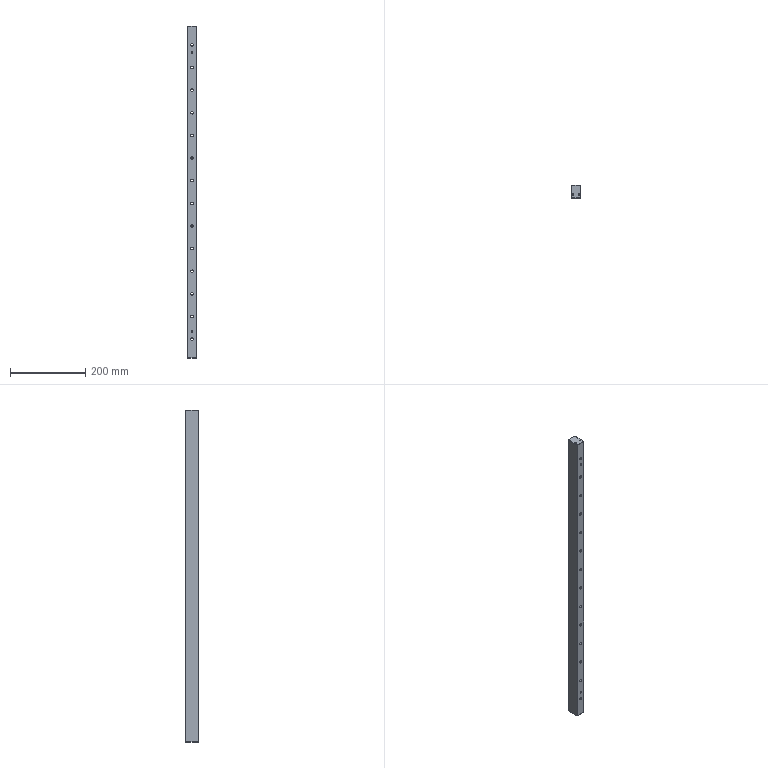Part | NX | 1 solid | 110 faces | box 25 x 35 x 880 mm | volume 742036 mm3 | cylinder 49 | plane 40 | cone 21 | commonest cylinder face diameters 4.2 x19 6.6 x14 11 x14 5 x2